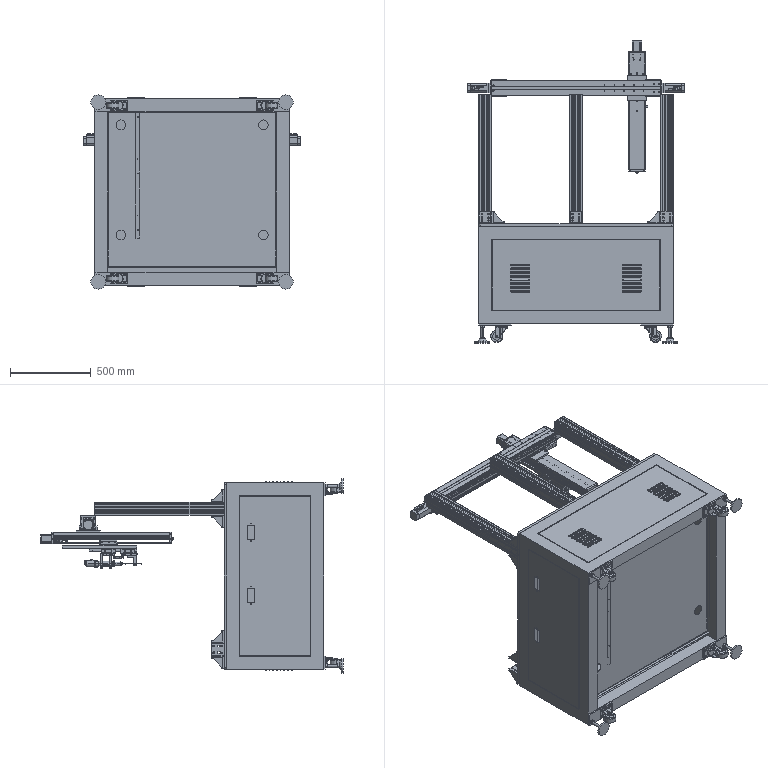Part | NX | 129 solids | 7404 faces | volume 110218188 mm3 | plane 3577 | cylinder 2304 | torus 570 | cone 464 | sphere 388 | spline 101 | commonest cylinder face diameters 10 x283 9 x270 6 x154 2 x138 12 x133 4 x122